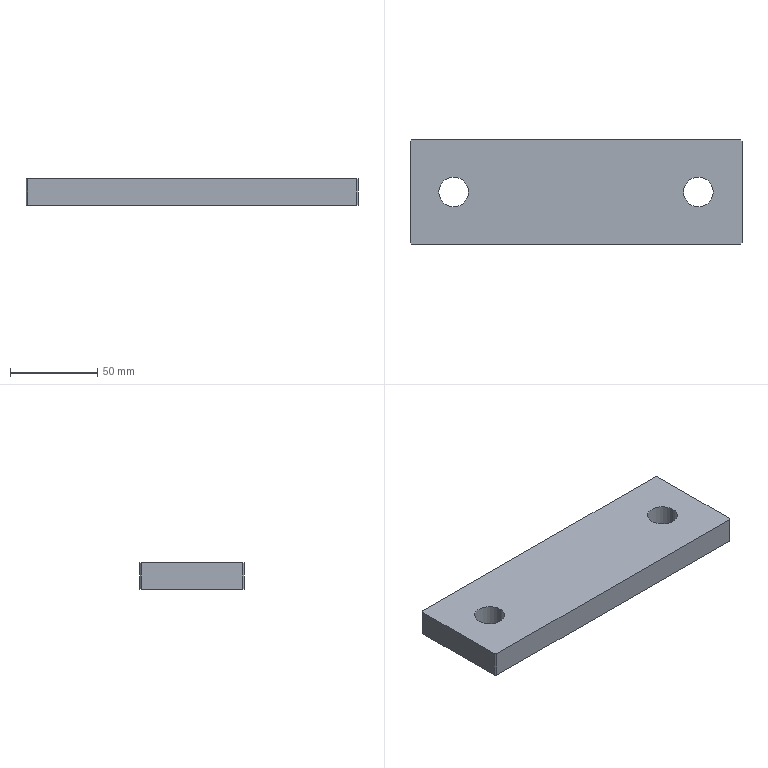Part | STEP file | Reinforcing plate | 1 solid | 14 faces | box 190 x 60 x 15 mm | volume 164161 mm3 | plane 10 | cylinder 4 | commonest cylinder face diameters 17 x4
STEP:
#1=CARTESIAN_POINT('',(0.,0.,0.));
#2=DIRECTION('',(0.,0.,1.));
#3=DIRECTION('',(1.,0.,0.));
#4=AXIS2_PLACEMENT_3D('',#1,#2,#3);
#5=CARTESIAN_POINT('',(516.5,-950.,15.));
#6=VERTEX_POINT('',#5);
#7=CARTESIAN_POINT('',(516.5,-950.,0.));
#8=VERTEX_POINT('',#7);
#9=CARTESIAN_POINT('',(516.5,-950.,0.));
#10=DIRECTION('',(0.,0.,-1.));
#11=VECTOR('',#10,1.);
#12=LINE('',#9,#11);
#13=CARTESIAN_POINT('',(525.,-950.,0.));
#14=DIRECTION('',(0.,0.,-1.));
#15=DIRECTION('',(-1.,0.,0.));
#16=AXIS2_PLACEMENT_3D('',#13,#14,#15);
#17=CYLINDRICAL_SURFACE('',#16,8.5);
#18=CARTESIAN_POINT('',(6.283,0.));
#19=DIRECTION('',(0.,1.));
#20=VECTOR('',#19,1.);
#21=LINE('',#18,#20);
#22=(GEOMETRIC_REPRESENTATION_CONTEXT(2)PARAMETRIC_REPRESENTATION_CONTEXT()REPRESENTATION_CONTEXT('',''));
#23=DEFINITIONAL_REPRESENTATION('',(#21),#22);
#24=PCURVE('',#17,#23);
#25=CARTESIAN_POINT('',(525.,-950.,0.));
#26=DIRECTION('',(0.,0.,-1.));
#27=DIRECTION('',(-1.,0.,0.));
#28=AXIS2_PLACEMENT_3D('',#25,#26,#27);
#29=CYLINDRICAL_SURFACE('',#28,8.5);
#30=CARTESIAN_POINT('',(0.,0.));
#31=DIRECTION('',(0.,1.));
#32=VECTOR('',#31,1.);
#33=LINE('',#30,#32);
#34=(GEOMETRIC_REPRESENTATION_CONTEXT(2)PARAMETRIC_REPRESENTATION_CONTEXT()REPRESENTATION_CONTEXT('',''));
#35=DEFINITIONAL_REPRESENTATION('',(#33),#34);
#36=PCURVE('',#29,#35);
#37=SURFACE_CURVE('',#12,(#24,#36),.PCURVE_S1.);
#38=EDGE_CURVE('',#6,#8,#37,.T.);
#39=ORIENTED_EDGE('',*,*,#38,.T.);
#40=CARTESIAN_POINT('',(533.5,-950.,0.));
#41=VERTEX_POINT('',#40);
#42=CARTESIAN_POINT('',(525.,-950.,0.));
#43=DIRECTION('',(0.,0.,-1.));
#44=DIRECTION('',(-1.,0.,0.));
#45=AXIS2_PLACEMENT_3D('',#42,#43,#44);
#46=CIRCLE('',#45,8.5);
#47=CARTESIAN_POINT('',(0.,0.));
#48=DIRECTION('',(1.,0.));
#49=VECTOR('',#48,1.);
#50=LINE('',#47,#49);
#51=(GEOMETRIC_REPRESENTATION_CONTEXT(2)PARAMETRIC_REPRESENTATION_CONTEXT()REPRESENTATION_CONTEXT('',''));
#52=DEFINITIONAL_REPRESENTATION('',(#50),#51);
#53=PCURVE('',#17,#52);
#54=CARTESIAN_POINT('',(0.,0.,0.));
#55=DIRECTION('',(0.,0.,1.));
#56=DIRECTION('',(1.,0.,0.));
#57=AXIS2_PLACEMENT_3D('',#54,#55,#56);
#58=PLANE('',#57);
#59=CARTESIAN_POINT('',(516.5,-950.));
#60=CARTESIAN_POINT('',(516.5,-935.278));
#61=CARTESIAN_POINT('',(529.25,-942.639));
#62=CARTESIAN_POINT('',(542.,-950.));
#63=CARTESIAN_POINT('',(529.25,-957.361));
#64=CARTESIAN_POINT('',(516.5,-964.722));
#65=CARTESIAN_POINT('',(516.5,-950.));
#66=(BOUNDED_CURVE()B_SPLINE_CURVE(2,(#59,#60,#61,#62,#63,#64,#65),.UNSPECIFIED.,.T.,.F.)B_SPLINE_CURVE_WITH_KNOTS((1,2,2,2,2,1),(-2.094,0.,2.094,4.189,6.283,8.378),.UNSPECIFIED.)CURVE()GEOMETRIC_REPRESENTATION_ITEM()RATIONAL_B_SPLINE_CURVE((1.,0.5,1.,0.5,1.,0.5,1.))REPRESENTATION_ITEM(''));
#67=(GEOMETRIC_REPRESENTATION_CONTEXT(2)PARAMETRIC_REPRESENTATION_CONTEXT()REPRESENTATION_CONTEXT('',''));
#68=DEFINITIONAL_REPRESENTATION('',(#66),#67);
#69=PCURVE('',#58,#68);
#70=SURFACE_CURVE('',#46,(#53,#69),.PCURVE_S1.);
#71=EDGE_CURVE('',#41,#8,#70,.T.);
#72=ORIENTED_EDGE('',*,*,#71,.F.);
#73=CARTESIAN_POINT('',(533.5,-950.,15.));
#74=VERTEX_POINT('',#73);
#75=CARTESIAN_POINT('',(533.5,-950.,0.));
#76=DIRECTION('',(0.,0.,-1.));
#77=VECTOR('',#76,1.);
#78=LINE('',#75,#77);
#79=CARTESIAN_POINT('',(3.142,0.));
#80=DIRECTION('',(0.,1.));
#81=VECTOR('',#80,1.);
#82=LINE('',#79,#81);
#83=(GEOMETRIC_REPRESENTATION_CONTEXT(2)PARAMETRIC_REPRESENTATION_CONTEXT()REPRESENTATION_CONTEXT('',''));
#84=DEFINITIONAL_REPRESENTATION('',(#82),#83);
#85=PCURVE('',#17,#84);
#86=CARTESIAN_POINT('',(3.142,0.));
#87=DIRECTION('',(0.,1.));
#88=VECTOR('',#87,1.);
#89=LINE('',#86,#88);
#90=(GEOMETRIC_REPRESENTATION_CONTEXT(2)PARAMETRIC_REPRESENTATION_CONTEXT()REPRESENTATION_CONTEXT('',''));
#91=DEFINITIONAL_REPRESENTATION('',(#89),#90);
#92=PCURVE('',#29,#91);
#93=SURFACE_CURVE('',#78,(#85,#92),.PCURVE_S1.);
#94=EDGE_CURVE('',#74,#41,#93,.T.);
#95=ORIENTED_EDGE('',*,*,#94,.F.);
#96=CARTESIAN_POINT('',(525.,-950.,15.));
#97=DIRECTION('',(0.,0.,-1.));
#98=DIRECTION('',(-1.,0.,0.));
#99=AXIS2_PLACEMENT_3D('',#96,#97,#98);
#100=CIRCLE('',#99,8.5);
#101=CARTESIAN_POINT('',(0.,-15.));
#102=DIRECTION('',(1.,0.));
#103=VECTOR('',#102,1.);
#104=LINE('',#101,#103);
#105=(GEOMETRIC_REPRESENTATION_CONTEXT(2)PARAMETRIC_REPRESENTATION_CONTEXT()REPRESENTATION_CONTEXT('',''));
#106=DEFINITIONAL_REPRESENTATION('',(#104),#105);
#107=PCURVE('',#17,#106);
#108=CARTESIAN_POINT('',(0.,0.,15.));
#109=DIRECTION('',(0.,0.,1.));
#110=DIRECTION('',(1.,0.,0.));
#111=AXIS2_PLACEMENT_3D('',#108,#109,#110);
#112=PLANE('',#111);
#113=CARTESIAN_POINT('',(516.5,-950.));
#114=CARTESIAN_POINT('',(516.5,-935.278));
#115=CARTESIAN_POINT('',(529.25,-942.639));
#116=CARTESIAN_POINT('',(542.,-950.));
#117=CARTESIAN_POINT('',(529.25,-957.361));
#118=CARTESIAN_POINT('',(516.5,-964.722));
#119=CARTESIAN_POINT('',(516.5,-950.));
#120=(BOUNDED_CURVE()B_SPLINE_CURVE(2,(#113,#114,#115,#116,#117,#118,#119),.UNSPECIFIED.,.T.,.F.)B_SPLINE_CURVE_WITH_KNOTS((1,2,2,2,2,1),(-2.094,0.,2.094,4.189,6.283,8.378),.UNSPECIFIED.)CURVE()GEOMETRIC_REPRESENTATION_ITEM()RATIONAL_B_SPLINE_CURVE((1.,0.5,1.,0.5,1.,0.5,1.))REPRESENTATION_ITEM(''));
#121=(GEOMETRIC_REPRESENTATION_CONTEXT(2)PARAMETRIC_REPRESENTATION_CONTEXT()REPRESENTATION_CONTEXT('',''));
#122=DEFINITIONAL_REPRESENTATION('',(#120),#121);
#123=PCURVE('',#112,#122);
#124=SURFACE_CURVE('',#100,(#107,#123),.PCURVE_S1.);
#125=EDGE_CURVE('',#74,#6,#124,.T.);
#126=ORIENTED_EDGE('',*,*,#125,.T.);
#127=EDGE_LOOP('',(#39,#72,#95,#126));
#128=FACE_BOUND('',#127,.F.);
#129=ADVANCED_FACE('',(#128),#17,.F.);
#130=CARTESIAN_POINT('',(376.5,-950.,15.));
#131=VERTEX_POINT('',#130);
#132=CARTESIAN_POINT('',(376.5,-950.,0.));
#133=VERTEX_POINT('',#132);
#134=CARTESIAN_POINT('',(376.5,-950.,0.));
#135=DIRECTION('',(0.,0.,-1.));
#136=VECTOR('',#135,1.);
#137=LINE('',#134,#136);
#138=CARTESIAN_POINT('',(385.,-950.,0.));
#139=DIRECTION('',(0.,0.,-1.));
#140=DIRECTION('',(-1.,0.,0.));
#141=AXIS2_PLACEMENT_3D('',#138,#139,#140);
#142=CYLINDRICAL_SURFACE('',#141,8.5);
#143=CARTESIAN_POINT('',(6.283,0.));
#144=DIRECTION('',(0.,1.));
#145=VECTOR('',#144,1.);
#146=LINE('',#143,#145);
#147=(GEOMETRIC_REPRESENTATION_CONTEXT(2)PARAMETRIC_REPRESENTATION_CONTEXT()REPRESENTATION_CONTEXT('',''));
#148=DEFINITIONAL_REPRESENTATION('',(#146),#147);
#149=PCURVE('',#142,#148);
#150=CARTESIAN_POINT('',(385.,-950.,0.));
#151=DIRECTION('',(0.,0.,-1.));
#152=DIRECTION('',(-1.,0.,0.));
#153=AXIS2_PLACEMENT_3D('',#150,#151,#152);
#154=CYLINDRICAL_SURFACE('',#153,8.5);
#155=CARTESIAN_POINT('',(0.,0.));
#156=DIRECTION('',(0.,1.));
#157=VECTOR('',#156,1.);
#158=LINE('',#155,#157);
#159=(GEOMETRIC_REPRESENTATION_CONTEXT(2)PARAMETRIC_REPRESENTATION_CONTEXT()REPRESENTATION_CONTEXT('',''));
#160=DEFINITIONAL_REPRESENTATION('',(#158),#159);
#161=PCURVE('',#154,#160);
#162=SURFACE_CURVE('',#137,(#149,#161),.PCURVE_S1.);
#163=EDGE_CURVE('',#131,#133,#162,.T.);
#164=ORIENTED_EDGE('',*,*,#163,.T.);
#165=CARTESIAN_POINT('',(393.5,-950.,0.));
#166=VERTEX_POINT('',#165);
#167=CARTESIAN_POINT('',(385.,-950.,0.));
#168=DIRECTION('',(0.,0.,-1.));
#169=DIRECTION('',(-1.,0.,0.));
#170=AXIS2_PLACEMENT_3D('',#167,#168,#169);
#171=CIRCLE('',#170,8.5);
#172=CARTESIAN_POINT('',(0.,0.));
#173=DIRECTION('',(1.,0.));
#174=VECTOR('',#173,1.);
#175=LINE('',#172,#174);
#176=(GEOMETRIC_REPRESENTATION_CONTEXT(2)PARAMETRIC_REPRESENTATION_CONTEXT()REPRESENTATION_CONTEXT('',''));
#177=DEFINITIONAL_REPRESENTATION('',(#175),#176);
#178=PCURVE('',#142,#177);
#179=CARTESIAN_POINT('',(376.5,-950.));
#180=CARTESIAN_POINT('',(376.5,-935.278));
#181=CARTESIAN_POINT('',(389.25,-942.639));
#182=CARTESIAN_POINT('',(402.,-950.));
#183=CARTESIAN_POINT('',(389.25,-957.361));
#184=CARTESIAN_POINT('',(376.5,-964.722));
#185=CARTESIAN_POINT('',(376.5,-950.));
#186=(BOUNDED_CURVE()B_SPLINE_CURVE(2,(#179,#180,#181,#182,#183,#184,#185),.UNSPECIFIED.,.T.,.F.)B_SPLINE_CURVE_WITH_KNOTS((1,2,2,2,2,1),(-2.094,0.,2.094,4.189,6.283,8.378),.UNSPECIFIED.)CURVE()GEOMETRIC_REPRESENTATION_ITEM()RATIONAL_B_SPLINE_CURVE((1.,0.5,1.,0.5,1.,0.5,1.))REPRESENTATION_ITEM(''));
#187=(GEOMETRIC_REPRESENTATION_CONTEXT(2)PARAMETRIC_REPRESENTATION_CONTEXT()REPRESENTATION_CONTEXT('',''));
#188=DEFINITIONAL_REPRESENTATION('',(#186),#187);
#189=PCURVE('',#58,#188);
#190=SURFACE_CURVE('',#171,(#178,#189),.PCURVE_S1.);
#191=EDGE_CURVE('',#166,#133,#190,.T.);
#192=ORIENTED_EDGE('',*,*,#191,.F.);
#193=CARTESIAN_POINT('',(393.5,-950.,15.));
#194=VERTEX_POINT('',#193);
#195=CARTESIAN_POINT('',(393.5,-950.,0.));
#196=DIRECTION('',(0.,0.,-1.));
#197=VECTOR('',#196,1.);
#198=LINE('',#195,#197);
#199=CARTESIAN_POINT('',(3.142,0.));
#200=DIRECTION('',(0.,1.));
#201=VECTOR('',#200,1.);
#202=LINE('',#199,#201);
#203=(GEOMETRIC_REPRESENTATION_CONTEXT(2)PARAMETRIC_REPRESENTATION_CONTEXT()REPRESENTATION_CONTEXT('',''));
#204=DEFINITIONAL_REPRESENTATION('',(#202),#203);
#205=PCURVE('',#142,#204);
#206=CARTESIAN_POINT('',(3.142,0.));
#207=DIRECTION('',(0.,1.));
#208=VECTOR('',#207,1.);
#209=LINE('',#206,#208);
#210=(GEOMETRIC_REPRESENTATION_CONTEXT(2)PARAMETRIC_REPRESENTATION_CONTEXT()REPRESENTATION_CONTEXT('',''));
#211=DEFINITIONAL_REPRESENTATION('',(#209),#210);
#212=PCURVE('',#154,#211);
#213=SURFACE_CURVE('',#198,(#205,#212),.PCURVE_S1.);
#214=EDGE_CURVE('',#194,#166,#213,.T.);
#215=ORIENTED_EDGE('',*,*,#214,.F.);
#216=CARTESIAN_POINT('',(385.,-950.,15.));
#217=DIRECTION('',(0.,0.,-1.));
#218=DIRECTION('',(-1.,0.,0.));
#219=AXIS2_PLACEMENT_3D('',#216,#217,#218);
#220=CIRCLE('',#219,8.5);
#221=CARTESIAN_POINT('',(0.,-15.));
#222=DIRECTION('',(1.,0.));
#223=VECTOR('',#222,1.);
#224=LINE('',#221,#223);
#225=(GEOMETRIC_REPRESENTATION_CONTEXT(2)PARAMETRIC_REPRESENTATION_CONTEXT()REPRESENTATION_CONTEXT('',''));
#226=DEFINITIONAL_REPRESENTATION('',(#224),#225);
#227=PCURVE('',#142,#226);
#228=CARTESIAN_POINT('',(376.5,-950.));
#229=CARTESIAN_POINT('',(376.5,-935.278));
#230=CARTESIAN_POINT('',(389.25,-942.639));
#231=CARTESIAN_POINT('',(402.,-950.));
#232=CARTESIAN_POINT('',(389.25,-957.361));
#233=CARTESIAN_POINT('',(376.5,-964.722));
#234=CARTESIAN_POINT('',(376.5,-950.));
#235=(BOUNDED_CURVE()B_SPLINE_CURVE(2,(#228,#229,#230,#231,#232,#233,#234),.UNSPECIFIED.,.T.,.F.)B_SPLINE_CURVE_WITH_KNOTS((1,2,2,2,2,1),(-2.094,0.,2.094,4.189,6.283,8.378),.UNSPECIFIED.)CURVE()GEOMETRIC_REPRESENTATION_ITEM()RATIONAL_B_SPLINE_CURVE((1.,0.5,1.,0.5,1.,0.5,1.))REPRESENTATION_ITEM(''));
#236=(GEOMETRIC_REPRESENTATION_CONTEXT(2)PARAMETRIC_REPRESENTATION_CONTEXT()REPRESENTATION_CONTEXT('',''));
#237=DEFINITIONAL_REPRESENTATION('',(#235),#236);
#238=PCURVE('',#112,#237);
#239=SURFACE_CURVE('',#220,(#227,#238),.PCURVE_S1.);
#240=EDGE_CURVE('',#194,#131,#239,.T.);
#241=ORIENTED_EDGE('',*,*,#240,.T.);
#242=EDGE_LOOP('',(#164,#192,#215,#241));
#243=FACE_BOUND('',#242,.F.);
#244=ADVANCED_FACE('',(#243),#142,.F.);
#245=CARTESIAN_POINT('',(360.,-921.,0.));
#246=VERTEX_POINT('',#245);
#247=CARTESIAN_POINT('',(360.,-979.,0.));
#248=VERTEX_POINT('',#247);
#249=CARTESIAN_POINT('',(360.,-980.,0.));
#250=DIRECTION('',(0.,-1.,0.));
#251=VECTOR('',#250,1.);
#252=LINE('',#249,#251);
#253=CARTESIAN_POINT('',(360.,-980.,15.));
#254=DIRECTION('',(1.,0.,0.));
#255=DIRECTION('',(0.,0.,-1.));
#256=AXIS2_PLACEMENT_3D('',#253,#254,#255);
#257=PLANE('',#256);
#258=CARTESIAN_POINT('',(15.,0.));
#259=DIRECTION('',(0.,-1.));
#260=VECTOR('',#259,1.);
#261=LINE('',#258,#260);
#262=(GEOMETRIC_REPRESENTATION_CONTEXT(2)PARAMETRIC_REPRESENTATION_CONTEXT()REPRESENTATION_CONTEXT('',''));
#263=DEFINITIONAL_REPRESENTATION('',(#261),#262);
#264=PCURVE('',#257,#263);
#265=CARTESIAN_POINT('',(360.,-980.));
#266=DIRECTION('',(0.,-1.));
#267=VECTOR('',#266,1.);
#268=LINE('',#265,#267);
#269=(GEOMETRIC_REPRESENTATION_CONTEXT(2)PARAMETRIC_REPRESENTATION_CONTEXT()REPRESENTATION_CONTEXT('',''));
#270=DEFINITIONAL_REPRESENTATION('',(#268),#269);
#271=PCURVE('',#58,#270);
#272=SURFACE_CURVE('',#252,(#264,#271),.PCURVE_S1.);
#273=EDGE_CURVE('',#246,#248,#272,.T.);
#274=ORIENTED_EDGE('',*,*,#273,.T.);
#275=CARTESIAN_POINT('',(360.,-979.,15.));
#276=VERTEX_POINT('',#275);
#277=CARTESIAN_POINT('',(360.,-979.,15.));
#278=DIRECTION('',(0.,0.,1.));
#279=VECTOR('',#278,1.);
#280=LINE('',#277,#279);
#281=CARTESIAN_POINT('',(0.,1.));
#282=DIRECTION('',(-1.,0.));
#283=VECTOR('',#282,1.);
#284=LINE('',#281,#283);
#285=(GEOMETRIC_REPRESENTATION_CONTEXT(2)PARAMETRIC_REPRESENTATION_CONTEXT()REPRESENTATION_CONTEXT('',''));
#286=DEFINITIONAL_REPRESENTATION('',(#284),#285);
#287=PCURVE('',#257,#286);
#288=CARTESIAN_POINT('',(361.,-980.,15.));
#289=DIRECTION('',(0.7071,0.7071,0.));
#290=DIRECTION('',(0.,0.,-1.));
#291=AXIS2_PLACEMENT_3D('',#288,#289,#290);
#292=PLANE('',#291);
#293=CARTESIAN_POINT('',(0.,1.414));
#294=DIRECTION('',(-1.,0.));
#295=VECTOR('',#294,1.);
#296=LINE('',#293,#295);
#297=(GEOMETRIC_REPRESENTATION_CONTEXT(2)PARAMETRIC_REPRESENTATION_CONTEXT()REPRESENTATION_CONTEXT('',''));
#298=DEFINITIONAL_REPRESENTATION('',(#296),#297);
#299=PCURVE('',#292,#298);
#300=SURFACE_CURVE('',#280,(#287,#299),.PCURVE_S1.);
#301=EDGE_CURVE('',#248,#276,#300,.T.);
#302=ORIENTED_EDGE('',*,*,#301,.T.);
#303=CARTESIAN_POINT('',(360.,-921.,15.));
#304=VERTEX_POINT('',#303);
#305=CARTESIAN_POINT('',(360.,-980.,15.));
#306=DIRECTION('',(0.,-1.,0.));
#307=VECTOR('',#306,1.);
#308=LINE('',#305,#307);
#309=CARTESIAN_POINT('',(0.,0.));
#310=DIRECTION('',(0.,-1.));
#311=VECTOR('',#310,1.);
#312=LINE('',#309,#311);
#313=(GEOMETRIC_REPRESENTATION_CONTEXT(2)PARAMETRIC_REPRESENTATION_CONTEXT()REPRESENTATION_CONTEXT('',''));
#314=DEFINITIONAL_REPRESENTATION('',(#312),#313);
#315=PCURVE('',#257,#314);
#316=CARTESIAN_POINT('',(360.,-980.));
#317=DIRECTION('',(0.,-1.));
#318=VECTOR('',#317,1.);
#319=LINE('',#316,#318);
#320=(GEOMETRIC_REPRESENTATION_CONTEXT(2)PARAMETRIC_REPRESENTATION_CONTEXT()REPRESENTATION_CONTEXT('',''));
#321=DEFINITIONAL_REPRESENTATION('',(#319),#320);
#322=PCURVE('',#112,#321);
#323=SURFACE_CURVE('',#308,(#315,#322),.PCURVE_S1.);
#324=EDGE_CURVE('',#304,#276,#323,.T.);
#325=ORIENTED_EDGE('',*,*,#324,.F.);
#326=CARTESIAN_POINT('',(360.,-921.,15.));
#327=DIRECTION('',(0.,0.,-1.));
#328=VECTOR('',#327,1.);
#329=LINE('',#326,#328);
#330=CARTESIAN_POINT('',(0.,59.));
#331=DIRECTION('',(1.,0.));
#332=VECTOR('',#331,1.);
#333=LINE('',#330,#332);
#334=(GEOMETRIC_REPRESENTATION_CONTEXT(2)PARAMETRIC_REPRESENTATION_CONTEXT()REPRESENTATION_CONTEXT('',''));
#335=DEFINITIONAL_REPRESENTATION('',(#333),#334);
#336=PCURVE('',#257,#335);
#337=CARTESIAN_POINT('',(360.,-921.,15.));
#338=DIRECTION('',(0.7071,-0.7071,0.));
#339=DIRECTION('',(0.,0.,-1.));
#340=AXIS2_PLACEMENT_3D('',#337,#338,#339);
#341=PLANE('',#340);
#342=CARTESIAN_POINT('',(0.,0.));
#343=DIRECTION('',(1.,0.));
#344=VECTOR('',#343,1.);
#345=LINE('',#342,#344);
#346=(GEOMETRIC_REPRESENTATION_CONTEXT(2)PARAMETRIC_REPRESENTATION_CONTEXT()REPRESENTATION_CONTEXT('',''));
#347=DEFINITIONAL_REPRESENTATION('',(#345),#346);
#348=PCURVE('',#341,#347);
#349=SURFACE_CURVE('',#329,(#336,#348),.PCURVE_S1.);
#350=EDGE_CURVE('',#304,#246,#349,.T.);
#351=ORIENTED_EDGE('',*,*,#350,.T.);
#352=EDGE_LOOP('',(#274,#302,#325,#351));
#353=FACE_BOUND('',#352,.T.);
#354=ADVANCED_FACE('',(#353),#257,.F.);
#355=CARTESIAN_POINT('',(361.,-980.,0.));
#356=VERTEX_POINT('',#355);
#357=CARTESIAN_POINT('',(549.,-980.,0.));
#358=VERTEX_POINT('',#357);
#359=CARTESIAN_POINT('',(550.,-980.,0.));
#360=DIRECTION('',(1.,0.,0.));
#361=VECTOR('',#360,1.);
#362=LINE('',#359,#361);
#363=CARTESIAN_POINT('',(550.,-980.,15.));
#364=DIRECTION('',(0.,1.,0.));
#365=DIRECTION('',(0.,0.,1.));
#366=AXIS2_PLACEMENT_3D('',#363,#364,#365);
#367=PLANE('',#366);
#368=CARTESIAN_POINT('',(-15.,0.));
#369=DIRECTION('',(0.,1.));
#370=VECTOR('',#369,1.);
#371=LINE('',#368,#370);
#372=(GEOMETRIC_REPRESENTATION_CONTEXT(2)PARAMETRIC_REPRESENTATION_CONTEXT()REPRESENTATION_CONTEXT('',''));
#373=DEFINITIONAL_REPRESENTATION('',(#371),#372);
#374=PCURVE('',#367,#373);
#375=CARTESIAN_POINT('',(550.,-980.));
#376=DIRECTION('',(1.,0.));
#377=VECTOR('',#376,1.);
#378=LINE('',#375,#377);
#379=(GEOMETRIC_REPRESENTATION_CONTEXT(2)PARAMETRIC_REPRESENTATION_CONTEXT()REPRESENTATION_CONTEXT('',''));
#380=DEFINITIONAL_REPRESENTATION('',(#378),#379);
#381=PCURVE('',#58,#380);
#382=SURFACE_CURVE('',#362,(#374,#381),.PCURVE_S1.);
#383=EDGE_CURVE('',#356,#358,#382,.T.);
#384=ORIENTED_EDGE('',*,*,#383,.T.);
#385=CARTESIAN_POINT('',(549.,-980.,15.));
#386=VERTEX_POINT('',#385);
#387=CARTESIAN_POINT('',(549.,-980.,15.));
#388=DIRECTION('',(0.,0.,1.));
#389=VECTOR('',#388,1.);
#390=LINE('',#387,#389);
#391=CARTESIAN_POINT('',(0.,-1.));
#392=DIRECTION('',(1.,0.));
#393=VECTOR('',#392,1.);
#394=LINE('',#391,#393);
#395=(GEOMETRIC_REPRESENTATION_CONTEXT(2)PARAMETRIC_REPRESENTATION_CONTEXT()REPRESENTATION_CONTEXT('',''));
#396=DEFINITIONAL_REPRESENTATION('',(#394),#395);
#397=PCURVE('',#367,#396);
#398=CARTESIAN_POINT('',(550.,-979.,15.));
#399=DIRECTION('',(-0.7071,0.7071,0.));
#400=DIRECTION('',(0.,0.,-1.));
#401=AXIS2_PLACEMENT_3D('',#398,#399,#400);
#402=PLANE('',#401);
#403=CARTESIAN_POINT('',(0.,1.414));
#404=DIRECTION('',(-1.,0.));
#405=VECTOR('',#404,1.);
#406=LINE('',#403,#405);
#407=(GEOMETRIC_REPRESENTATION_CONTEXT(2)PARAMETRIC_REPRESENTATION_CONTEXT()REPRESENTATION_CONTEXT('',''));
#408=DEFINITIONAL_REPRESENTATION('',(#406),#407);
#409=PCURVE('',#402,#408);
#410=SURFACE_CURVE('',#390,(#397,#409),.PCURVE_S1.);
#411=EDGE_CURVE('',#358,#386,#410,.T.);
#412=ORIENTED_EDGE('',*,*,#411,.T.);
#413=CARTESIAN_POINT('',(361.,-980.,15.));
#414=VERTEX_POINT('',#413);
#415=CARTESIAN_POINT('',(550.,-980.,15.));
#416=DIRECTION('',(1.,0.,0.));
#417=VECTOR('',#416,1.);
#418=LINE('',#415,#417);
#419=CARTESIAN_POINT('',(0.,0.));
#420=DIRECTION('',(0.,1.));
#421=VECTOR('',#420,1.);
#422=LINE('',#419,#421);
#423=(GEOMETRIC_REPRESENTATION_CONTEXT(2)PARAMETRIC_REPRESENTATION_CONTEXT()REPRESENTATION_CONTEXT('',''));
#424=DEFINITIONAL_REPRESENTATION('',(#422),#423);
#425=PCURVE('',#367,#424);
#426=CARTESIAN_POINT('',(550.,-980.));
#427=DIRECTION('',(1.,0.));
#428=VECTOR('',#427,1.);
#429=LINE('',#426,#428);
#430=(GEOMETRIC_REPRESENTATION_CONTEXT(2)PARAMETRIC_REPRESENTATION_CONTEXT()REPRESENTATION_CONTEXT('',''));
#431=DEFINITIONAL_REPRESENTATION('',(#429),#430);
#432=PCURVE('',#112,#431);
#433=SURFACE_CURVE('',#418,(#425,#432),.PCURVE_S1.);
#434=EDGE_CURVE('',#414,#386,#433,.T.);
#435=ORIENTED_EDGE('',*,*,#434,.F.);
#436=CARTESIAN_POINT('',(361.,-980.,15.));
#437=DIRECTION('',(0.,0.,-1.));
#438=VECTOR('',#437,1.);
#439=LINE('',#436,#438);
#440=CARTESIAN_POINT('',(0.,-189.));
#441=DIRECTION('',(-1.,0.));
#442=VECTOR('',#441,1.);
#443=LINE('',#440,#442);
#444=(GEOMETRIC_REPRESENTATION_CONTEXT(2)PARAMETRIC_REPRESENTATION_CONTEXT()REPRESENTATION_CONTEXT('',''));
#445=DEFINITIONAL_REPRESENTATION('',(#443),#444);
#446=PCURVE('',#367,#445);
#447=CARTESIAN_POINT('',(0.,0.));
#448=DIRECTION('',(1.,0.));
#449=VECTOR('',#448,1.);
#450=LINE('',#447,#449);
#451=(GEOMETRIC_REPRESENTATION_CONTEXT(2)PARAMETRIC_REPRESENTATION_CONTEXT()REPRESENTATION_CONTEXT('',''));
#452=DEFINITIONAL_REPRESENTATION('',(#450),#451);
#453=PCURVE('',#292,#452);
#454=SURFACE_CURVE('',#439,(#446,#453),.PCURVE_S1.);
#455=EDGE_CURVE('',#414,#356,#454,.T.);
#456=ORIENTED_EDGE('',*,*,#455,.T.);
#457=EDGE_LOOP('',(#384,#412,#435,#456));
#458=FACE_BOUND('',#457,.T.);
#459=ADVANCED_FACE('',(#458),#367,.F.);
#460=CARTESIAN_POINT('',(550.,-979.,15.));
#461=VERTEX_POINT('',#460);
#462=CARTESIAN_POINT('',(550.,-921.,15.));
#463=VERTEX_POINT('',#462);
#464=CARTESIAN_POINT('',(550.,-980.,15.));
#465=DIRECTION('',(0.,1.,0.));
#466=VECTOR('',#465,1.);
#467=LINE('',#464,#466);
#468=CARTESIAN_POINT('',(550.,-980.,15.));
#469=DIRECTION('',(-1.,0.,0.));
#470=DIRECTION('',(0.,0.,1.));
#471=AXIS2_PLACEMENT_3D('',#468,#469,#470);
#472=PLANE('',#471);
#473=CARTESIAN_POINT('',(0.,0.));
#474=DIRECTION('',(0.,1.));
#475=VECTOR('',#474,1.);
#476=LINE('',#473,#475);
#477=(GEOMETRIC_REPRESENTATION_CONTEXT(2)PARAMETRIC_REPRESENTATION_CONTEXT()REPRESENTATION_CONTEXT('',''));
#478=DEFINITIONAL_REPRESENTATION('',(#476),#477);
#479=PCURVE('',#472,#478);
#480=CARTESIAN_POINT('',(550.,-980.));
#481=DIRECTION('',(0.,1.));
#482=VECTOR('',#481,1.);
#483=LINE('',#480,#482);
#484=(GEOMETRIC_REPRESENTATION_CONTEXT(2)PARAMETRIC_REPRESENTATION_CONTEXT()REPRESENTATION_CONTEXT('',''));
#485=DEFINITIONAL_REPRESENTATION('',(#483),#484);
#486=PCURVE('',#112,#485);
#487=SURFACE_CURVE('',#467,(#479,#486),.PCURVE_S1.);
#488=EDGE_CURVE('',#461,#463,#487,.T.);
#489=ORIENTED_EDGE('',*,*,#488,.F.);
#490=CARTESIAN_POINT('',(550.,-979.,0.));
#491=VERTEX_POINT('',#490);
#492=CARTESIAN_POINT('',(550.,-979.,15.));
#493=DIRECTION('',(0.,0.,-1.));
#494=VECTOR('',#493,1.);
#495=LINE('',#492,#494);
#496=CARTESIAN_POINT('',(0.,1.));
#497=DIRECTION('',(-1.,0.));
#498=VECTOR('',#497,1.);
#499=LINE('',#496,#498);
#500=(GEOMETRIC_REPRESENTATION_CONTEXT(2)PARAMETRIC_REPRESENTATION_CONTEXT()REPRESENTATION_CONTEXT('',''));
#501=DEFINITIONAL_REPRESENTATION('',(#499),#500);
#502=PCURVE('',#472,#501);
#503=CARTESIAN_POINT('',(0.,0.));
#504=DIRECTION('',(1.,0.));
#505=VECTOR('',#504,1.);
#506=LINE('',#503,#505);
#507=(GEOMETRIC_REPRESENTATION_CONTEXT(2)PARAMETRIC_REPRESENTATION_CONTEXT()REPRESENTATION_CONTEXT('',''));
#508=DEFINITIONAL_REPRESENTATION('',(#506),#507);
#509=PCURVE('',#402,#508);
#510=SURFACE_CURVE('',#495,(#502,#509),.PCURVE_S1.);
#511=EDGE_CURVE('',#461,#491,#510,.T.);
#512=ORIENTED_EDGE('',*,*,#511,.T.);
#513=CARTESIAN_POINT('',(550.,-921.,0.));
#514=VERTEX_POINT('',#513);
#515=CARTESIAN_POINT('',(550.,-980.,0.));
#516=DIRECTION('',(0.,1.,0.));
#517=VECTOR('',#516,1.);
#518=LINE('',#515,#517);
#519=CARTESIAN_POINT('',(-15.,0.));
#520=DIRECTION('',(0.,1.));
#521=VECTOR('',#520,1.);
#522=LINE('',#519,#521);
#523=(GEOMETRIC_REPRESENTATION_CONTEXT(2)PARAMETRIC_REPRESENTATION_CONTEXT()REPRESENTATION_CONTEXT('',''));
#524=DEFINITIONAL_REPRESENTATION('',(#522),#523);
#525=PCURVE('',#472,#524);
#526=CARTESIAN_POINT('',(550.,-980.));
#527=DIRECTION('',(0.,1.));
#528=VECTOR('',#527,1.);
#529=LINE('',#526,#528);
#530=(GEOMETRIC_REPRESENTATION_CONTEXT(2)PARAMETRIC_REPRESENTATION_CONTEXT()REPRESENTATION_CONTEXT('',''));
#531=DEFINITIONAL_REPRESENTATION('',(#529),#530);
#532=PCURVE('',#58,#531);
#533=SURFACE_CURVE('',#518,(#525,#532),.PCURVE_S1.);
#534=EDGE_CURVE('',#491,#514,#533,.T.);
#535=ORIENTED_EDGE('',*,*,#534,.T.);
#536=CARTESIAN_POINT('',(550.,-921.,15.));
#537=DIRECTION('',(0.,0.,1.));
#538=VECTOR('',#537,1.);
#539=LINE('',#536,#538);
#540=CARTESIAN_POINT('',(0.,59.));
#541=DIRECTION('',(1.,0.));
#542=VECTOR('',#541,1.);
#543=LINE('',#540,#542);
#544=(GEOMETRIC_REPRESENTATION_CONTEXT(2)PARAMETRIC_REPRESENTATION_CONTEXT()REPRESENTATION_CONTEXT('',''));
#545=DEFINITIONAL_REPRESENTATION('',(#543),#544);
#546=PCURVE('',#472,#545);
#547=CARTESIAN_POINT('',(549.,-920.,15.));
#548=DIRECTION('',(-0.7071,-0.7071,0.));
#549=DIRECTION('',(0.,0.,-1.));
#550=AXIS2_PLACEMENT_3D('',#547,#548,#549);
#551=PLANE('',#550);
#552=CARTESIAN_POINT('',(0.,1.414));
#553=DIRECTION('',(-1.,0.));
#554=VECTOR('',#553,1.);
#555=LINE('',#552,#554);
#556=(GEOMETRIC_REPRESENTATION_CONTEXT(2)PARAMETRIC_REPRESENTATION_CONTEXT()REPRESENTATION_CONTEXT('',''));
#557=DEFINITIONAL_REPRESENTATION('',(#555),#556);
#558=PCURVE('',#551,#557);
#559=SURFACE_CURVE('',#539,(#546,#558),.PCURVE_S1.);
#560=EDGE_CURVE('',#514,#463,#559,.T.);
#561=ORIENTED_EDGE('',*,*,#560,.T.);
#562=EDGE_LOOP('',(#489,#512,#535,#561));
#563=FACE_BOUND('',#562,.T.);
#564=ADVANCED_FACE('',(#563),#472,.F.);
#565=CARTESIAN_POINT('',(549.,-920.,15.));
#566=VERTEX_POINT('',#565);
#567=CARTESIAN_POINT('',(361.,-920.,15.));
#568=VERTEX_POINT('',#567);
#569=CARTESIAN_POINT('',(550.,-920.,15.));
#570=DIRECTION('',(-1.,0.,0.));
#571=VECTOR('',#570,1.);
#572=LINE('',#569,#571);
#573=CARTESIAN_POINT('',(550.,-920.,15.));
#574=DIRECTION('',(0.,-1.,0.));
#575=DIRECTION('',(0.,0.,-1.));
#576=AXIS2_PLACEMENT_3D('',#573,#574,#575);
#577=PLANE('',#576);
#578=CARTESIAN_POINT('',(0.,0.));
#579=DIRECTION('',(0.,-1.));
#580=VECTOR('',#579,1.);
#581=LINE('',#578,#580);
#582=(GEOMETRIC_REPRESENTATION_CONTEXT(2)PARAMETRIC_REPRESENTATION_CONTEXT()REPRESENTATION_CONTEXT('',''));
#583=DEFINITIONAL_REPRESENTATION('',(#581),#582);
#584=PCURVE('',#577,#583);
#585=CARTESIAN_POINT('',(550.,-920.));
#586=DIRECTION('',(-1.,0.));
#587=VECTOR('',#586,1.);
#588=LINE('',#585,#587);
#589=(GEOMETRIC_REPRESENTATION_CONTEXT(2)PARAMETRIC_REPRESENTATION_CONTEXT()REPRESENTATION_CONTEXT('',''));
#590=DEFINITIONAL_REPRESENTATION('',(#588),#589);
#591=PCURVE('',#112,#590);
#592=SURFACE_CURVE('',#572,(#584,#591),.PCURVE_S1.);
#593=EDGE_CURVE('',#566,#568,#592,.T.);
#594=ORIENTED_EDGE('',*,*,#593,.F.);
#595=CARTESIAN_POINT('',(549.,-920.,0.));
#596=VERTEX_POINT('',#595);
#597=CARTESIAN_POINT('',(549.,-920.,15.));
#598=DIRECTION('',(0.,0.,-1.));
#599=VECTOR('',#598,1.);
#600=LINE('',#597,#599);
#601=CARTESIAN_POINT('',(0.,-1.));
#602=DIRECTION('',(1.,0.));
#603=VECTOR('',#602,1.);
#604=LINE('',#601,#603);
#605=(GEOMETRIC_REPRESENTATION_CONTEXT(2)PARAMETRIC_REPRESENTATION_CONTEXT()REPRESENTATION_CONTEXT('',''));
#606=DEFINITIONAL_REPRESENTATION('',(#604),#605);
#607=PCURVE('',#577,#606);
#608=CARTESIAN_POINT('',(0.,0.));
#609=DIRECTION('',(1.,0.));
#610=VECTOR('',#609,1.);
#611=LINE('',#608,#610);
#612=(GEOMETRIC_REPRESENTATION_CONTEXT(2)PARAMETRIC_REPRESENTATION_CONTEXT()REPRESENTATION_CONTEXT('',''));
#613=DEFINITIONAL_REPRESENTATION('',(#611),#612);
#614=PCURVE('',#551,#613);
#615=SURFACE_CURVE('',#600,(#607,#614),.PCURVE_S1.);
#616=EDGE_CURVE('',#566,#596,#615,.T.);
#617=ORIENTED_EDGE('',*,*,#616,.T.);
#618=CARTESIAN_POINT('',(361.,-920.,0.));
#619=VERTEX_POINT('',#618);
#620=CARTESIAN_POINT('',(550.,-920.,0.));
#621=DIRECTION('',(-1.,0.,0.));
#622=VECTOR('',#621,1.);
#623=LINE('',#620,#622);
#624=CARTESIAN_POINT('',(15.,0.));
#625=DIRECTION('',(0.,-1.));
#626=VECTOR('',#625,1.);
#627=LINE('',#624,#626);
#628=(GEOMETRIC_REPRESENTATION_CONTEXT(2)PARAMETRIC_REPRESENTATION_CONTEXT()REPRESENTATION_CONTEXT('',''));
#629=DEFINITIONAL_REPRESENTATION('',(#627),#628);
#630=PCURVE('',#577,#629);
#631=CARTESIAN_POINT('',(550.,-920.));
#632=DIRECTION('',(-1.,0.));
#633=VECTOR('',#632,1.);
#634=LINE('',#631,#633);
#635=(GEOMETRIC_REPRESENTATION_CONTEXT(2)PARAMETRIC_REPRESENTATION_CONTEXT()REPRESENTATION_CONTEXT('',''));
#636=DEFINITIONAL_REPRESENTATION('',(#634),#635);
#637=PCURVE('',#58,#636);
#638=SURFACE_CURVE('',#623,(#630,#637),.PCURVE_S1.);
#639=EDGE_CURVE('',#596,#619,#638,.T.);
#640=ORIENTED_EDGE('',*,*,#639,.T.);
#641=CARTESIAN_POINT('',(361.,-920.,15.));
#642=DIRECTION('',(0.,0.,1.));
#643=VECTOR('',#642,1.);
#644=LINE('',#641,#643);
#645=CARTESIAN_POINT('',(0.,-189.));
#646=DIRECTION('',(-1.,0.));
#647=VECTOR('',#646,1.);
#648=LINE('',#645,#647);
#649=(GEOMETRIC_REPRESENTATION_CONTEXT(2)PARAMETRIC_REPRESENTATION_CONTEXT()REPRESENTATION_CONTEXT('',''));
#650=DEFINITIONAL_REPRESENTATION('',(#648),#649);
#651=PCURVE('',#577,#650);
#652=CARTESIAN_POINT('',(0.,1.414));
#653=DIRECTION('',(-1.,0.));
#654=VECTOR('',#653,1.);
#655=LINE('',#652,#654);
#656=(GEOMETRIC_REPRESENTATION_CONTEXT(2)PARAMETRIC_REPRESENTATION_CONTEXT()REPRESENTATION_CONTEXT('',''));
#657=DEFINITIONAL_REPRESENTATION('',(#655),#656);
#658=PCURVE('',#341,#657);
#659=SURFACE_CURVE('',#644,(#651,#658),.PCURVE_S1.);
#660=EDGE_CURVE('',#619,#568,#659,.T.);
#661=ORIENTED_EDGE('',*,*,#660,.T.);
#662=EDGE_LOOP('',(#594,#617,#640,#661));
#663=FACE_BOUND('',#662,.T.);
#664=ADVANCED_FACE('',(#663),#577,.F.);
#665=CARTESIAN_POINT('',(525.,-950.,15.));
#666=DIRECTION('',(0.,0.,-1.));
#667=DIRECTION('',(-1.,0.,0.));
#668=AXIS2_PLACEMENT_3D('',#665,#666,#667);
#669=CIRCLE('',#668,8.5);
#670=CARTESIAN_POINT('',(516.5,-950.));
#671=CARTESIAN_POINT('',(516.5,-935.278));
#672=CARTESIAN_POINT('',(529.25,-942.639));
#673=CARTESIAN_POINT('',(542.,-950.));
#674=CARTESIAN_POINT('',(529.25,-957.361));
#675=CARTESIAN_POINT('',(516.5,-964.722));
#676=CARTESIAN_POINT('',(516.5,-950.));
#677=(BOUNDED_CURVE()B_SPLINE_CURVE(2,(#670,#671,#672,#673,#674,#675,#676),.UNSPECIFIED.,.T.,.F.)B_SPLINE_CURVE_WITH_KNOTS((1,2,2,2,2,1),(-2.094,0.,2.094,4.189,6.283,8.378),.UNSPECIFIED.)CURVE()GEOMETRIC_REPRESENTATION_ITEM()RATIONAL_B_SPLINE_CURVE((1.,0.5,1.,0.5,1.,0.5,1.))REPRESENTATION_ITEM(''));
#678=(GEOMETRIC_REPRESENTATION_CONTEXT(2)PARAMETRIC_REPRESENTATION_CONTEXT()REPRESENTATION_CONTEXT('',''));
#679=DEFINITIONAL_REPRESENTATION('',(#677),#678);
#680=PCURVE('',#112,#679);
#681=CARTESIAN_POINT('',(0.,-15.));
#682=DIRECTION('',(1.,0.));
#683=VECTOR('',#682,1.);
#684=LINE('',#681,#683);
#685=(GEOMETRIC_REPRESENTATION_CONTEXT(2)PARAMETRIC_REPRESENTATION_CONTEXT()REPRESENTATION_CONTEXT('',''));
#686=DEFINITIONAL_REPRESENTATION('',(#684),#685);
#687=PCURVE('',#29,#686);
#688=SURFACE_CURVE('',#669,(#680,#687),.PCURVE_S1.);
#689=EDGE_CURVE('',#6,#74,#688,.T.);
#690=ORIENTED_EDGE('',*,*,#689,.T.);
#691=ORIENTED_EDGE('',*,*,#125,.T.);
#692=EDGE_LOOP('',(#690,#691));
#693=FACE_BOUND('',#692,.T.);
#694=CARTESIAN_POINT('',(385.,-950.,15.));
#695=DIRECTION('',(0.,0.,-1.));
#696=DIRECTION('',(-1.,0.,0.));
#697=AXIS2_PLACEMENT_3D('',#694,#695,#696);
#698=CIRCLE('',#697,8.5);
#699=CARTESIAN_POINT('',(376.5,-950.));
#700=CARTESIAN_POINT('',(376.5,-935.278));
#701=CARTESIAN_POINT('',(389.25,-942.639));
#702=CARTESIAN_POINT('',(402.,-950.));
#703=CARTESIAN_POINT('',(389.25,-957.361));
#704=CARTESIAN_POINT('',(376.5,-964.722));
#705=CARTESIAN_POINT('',(376.5,-950.));
#706=(BOUNDED_CURVE()B_SPLINE_CURVE(2,(#699,#700,#701,#702,#703,#704,#705),.UNSPECIFIED.,.T.,.F.)B_SPLINE_CURVE_WITH_KNOTS((1,2,2,2,2,1),(-2.094,0.,2.094,4.189,6.283,8.378),.UNSPECIFIED.)CURVE()GEOMETRIC_REPRESENTATION_ITEM()RATIONAL_B_SPLINE_CURVE((1.,0.5,1.,0.5,1.,0.5,1.))REPRESENTATION_ITEM(''));
#707=(GEOMETRIC_REPRESENTATION_CONTEXT(2)PARAMETRIC_REPRESENTATION_CONTEXT()REPRESENTATION_CONTEXT('',''));
#708=DEFINITIONAL_REPRESENTATION('',(#706),#707);
#709=PCURVE('',#112,#708);
#710=CARTESIAN_POINT('',(0.,-15.));
#711=DIRECTION('',(1.,0.));
#712=VECTOR('',#711,1.);
#713=LINE('',#710,#712);
#714=(GEOMETRIC_REPRESENTATION_CONTEXT(2)PARAMETRIC_REPRESENTATION_CONTEXT()REPRESENTATION_CONTEXT('',''));
#715=DEFINITIONAL_REPRESENTATION('',(#713),#714);
#716=PCURVE('',#154,#715);
#717=SURFACE_CURVE('',#698,(#709,#716),.PCURVE_S1.);
#718=EDGE_CURVE('',#131,#194,#717,.T.);
#719=ORIENTED_EDGE('',*,*,#718,.T.);
#720=ORIENTED_EDGE('',*,*,#240,.T.);
#721=EDGE_LOOP('',(#719,#720));
#722=FACE_BOUND('',#721,.T.);
#723=ORIENTED_EDGE('',*,*,#434,.T.);
#724=CARTESIAN_POINT('',(764.5,-764.5,15.));
#725=DIRECTION('',(0.7071,0.7071,0.));
#726=VECTOR('',#725,1.);
#727=LINE('',#724,#726);
#728=CARTESIAN_POINT('',(764.5,-764.5));
#729=DIRECTION('',(0.7071,0.7071));
#730=VECTOR('',#729,1.);
#731=LINE('',#728,#730);
#732=(GEOMETRIC_REPRESENTATION_CONTEXT(2)PARAMETRIC_REPRESENTATION_CONTEXT()REPRESENTATION_CONTEXT('',''));
#733=DEFINITIONAL_REPRESENTATION('',(#731),#732);
#734=PCURVE('',#112,#733);
#735=CARTESIAN_POINT('',(0.,-303.349));
#736=DIRECTION('',(0.,-1.));
#737=VECTOR('',#736,1.);
#738=LINE('',#735,#737);
#739=(GEOMETRIC_REPRESENTATION_CONTEXT(2)PARAMETRIC_REPRESENTATION_CONTEXT()REPRESENTATION_CONTEXT('',''));
#740=DEFINITIONAL_REPRESENTATION('',(#738),#739);
#741=PCURVE('',#402,#740);
#742=SURFACE_CURVE('',#727,(#734,#741),.PCURVE_S1.);
#743=EDGE_CURVE('',#386,#461,#742,.T.);
#744=ORIENTED_EDGE('',*,*,#743,.T.);
#745=ORIENTED_EDGE('',*,*,#488,.T.);
#746=CARTESIAN_POINT('',(-185.5,-185.5,15.));
#747=DIRECTION('',(-0.7071,0.7071,0.));
#748=VECTOR('',#747,1.);
#749=LINE('',#746,#748);
#750=CARTESIAN_POINT('',(-185.5,-185.5));
#751=DIRECTION('',(-0.7071,0.7071));
#752=VECTOR('',#751,1.);
#753=LINE('',#750,#752);
#754=(GEOMETRIC_REPRESENTATION_CONTEXT(2)PARAMETRIC_REPRESENTATION_CONTEXT()REPRESENTATION_CONTEXT('',''));
#755=DEFINITIONAL_REPRESENTATION('',(#753),#754);
#756=PCURVE('',#112,#755);
#757=CARTESIAN_POINT('',(0.,-1038.74));
#758=DIRECTION('',(0.,-1.));
#759=VECTOR('',#758,1.);
#760=LINE('',#757,#759);
#761=(GEOMETRIC_REPRESENTATION_CONTEXT(2)PARAMETRIC_REPRESENTATION_CONTEXT()REPRESENTATION_CONTEXT('',''));
#762=DEFINITIONAL_REPRESENTATION('',(#760),#761);
#763=PCURVE('',#551,#762);
#764=SURFACE_CURVE('',#749,(#756,#763),.PCURVE_S1.);
#765=EDGE_CURVE('',#463,#566,#764,.T.);
#766=ORIENTED_EDGE('',*,*,#765,.T.);
#767=ORIENTED_EDGE('',*,*,#593,.T.);
#768=CARTESIAN_POINT('',(640.5,-640.5,15.));
#769=DIRECTION('',(-0.7071,-0.7071,0.));
#770=VECTOR('',#769,1.);
#771=LINE('',#768,#770);
#772=CARTESIAN_POINT('',(640.5,-640.5));
#773=DIRECTION('',(-0.7071,-0.7071));
#774=VECTOR('',#773,1.);
#775=LINE('',#772,#774);
#776=(GEOMETRIC_REPRESENTATION_CONTEXT(2)PARAMETRIC_REPRESENTATION_CONTEXT()REPRESENTATION_CONTEXT('',''));
#777=DEFINITIONAL_REPRESENTATION('',(#775),#776);
#778=PCURVE('',#112,#777);
#779=CARTESIAN_POINT('',(0.,396.687));
#780=DIRECTION('',(0.,-1.));
#781=VECTOR('',#780,1.);
#782=LINE('',#779,#781);
#783=(GEOMETRIC_REPRESENTATION_CONTEXT(2)PARAMETRIC_REPRESENTATION_CONTEXT()REPRESENTATION_CONTEXT('',''));
#784=DEFINITIONAL_REPRESENTATION('',(#782),#783);
#785=PCURVE('',#341,#784);
#786=SURFACE_CURVE('',#771,(#778,#785),.PCURVE_S1.);
#787=EDGE_CURVE('',#568,#304,#786,.T.);
#788=ORIENTED_EDGE('',*,*,#787,.T.);
#789=ORIENTED_EDGE('',*,*,#324,.T.);
#790=CARTESIAN_POINT('',(-309.5,-309.5,15.));
#791=DIRECTION('',(0.7071,-0.7071,0.));
#792=VECTOR('',#791,1.);
#793=LINE('',#790,#792);
#794=CARTESIAN_POINT('',(-309.5,-309.5));
#795=DIRECTION('',(0.7071,-0.7071));
#796=VECTOR('',#795,1.);
#797=LINE('',#794,#796);
#798=(GEOMETRIC_REPRESENTATION_CONTEXT(2)PARAMETRIC_REPRESENTATION_CONTEXT()REPRESENTATION_CONTEXT('',''));
#799=DEFINITIONAL_REPRESENTATION('',(#797),#798);
#800=PCURVE('',#112,#799);
#801=CARTESIAN_POINT('',(0.,948.23));
#802=DIRECTION('',(0.,-1.));
#803=VECTOR('',#802,1.);
#804=LINE('',#801,#803);
#805=(GEOMETRIC_REPRESENTATION_CONTEXT(2)PARAMETRIC_REPRESENTATION_CONTEXT()REPRESENTATION_CONTEXT('',''));
#806=DEFINITIONAL_REPRESENTATION('',(#804),#805);
#807=PCURVE('',#292,#806);
#808=SURFACE_CURVE('',#793,(#800,#807),.PCURVE_S1.);
#809=EDGE_CURVE('',#276,#414,#808,.T.);
#810=ORIENTED_EDGE('',*,*,#809,.T.);
#811=EDGE_LOOP('',(#723,#744,#745,#766,#767,#788,#789,#810));
#812=FACE_BOUND('',#811,.T.);
#813=ADVANCED_FACE('',(#693,#722,#812),#112,.T.);
#814=CARTESIAN_POINT('',(525.,-950.,0.));
#815=DIRECTION('',(0.,0.,-1.));
#816=DIRECTION('',(-1.,0.,0.));
#817=AXIS2_PLACEMENT_3D('',#814,#815,#816);
#818=CIRCLE('',#817,8.5);
#819=CARTESIAN_POINT('',(516.5,-950.));
#820=CARTESIAN_POINT('',(516.5,-935.278));
#821=CARTESIAN_POINT('',(529.25,-942.639));
#822=CARTESIAN_POINT('',(542.,-950.));
#823=CARTESIAN_POINT('',(529.25,-957.361));
#824=CARTESIAN_POINT('',(516.5,-964.722));
#825=CARTESIAN_POINT('',(516.5,-950.));
#826=(BOUNDED_CURVE()B_SPLINE_CURVE(2,(#819,#820,#821,#822,#823,#824,#825),.UNSPECIFIED.,.T.,.F.)B_SPLINE_CURVE_WITH_KNOTS((1,2,2,2,2,1),(-2.094,0.,2.094,4.189,6.283,8.378),.UNSPECIFIED.)CURVE()GEOMETRIC_REPRESENTATION_ITEM()RATIONAL_B_SPLINE_CURVE((1.,0.5,1.,0.5,1.,0.5,1.))REPRESENTATION_ITEM(''));
#827=(GEOMETRIC_REPRESENTATION_CONTEXT(2)PARAMETRIC_REPRESENTATION_CONTEXT()REPRESENTATION_CONTEXT('',''));
#828=DEFINITIONAL_REPRESENTATION('',(#826),#827);
#829=PCURVE('',#58,#828);
#830=CARTESIAN_POINT('',(0.,0.));
#831=DIRECTION('',(1.,0.));
#832=VECTOR('',#831,1.);
#833=LINE('',#830,#832);
#834=(GEOMETRIC_REPRESENTATION_CONTEXT(2)PARAMETRIC_REPRESENTATION_CONTEXT()REPRESENTATION_CONTEXT('',''));
#835=DEFINITIONAL_REPRESENTATION('',(#833),#834);
#836=PCURVE('',#29,#835);
#837=SURFACE_CURVE('',#818,(#829,#836),.PCURVE_S1.);
#838=EDGE_CURVE('',#8,#41,#837,.T.);
#839=ORIENTED_EDGE('',*,*,#838,.F.);
#840=ORIENTED_EDGE('',*,*,#71,.F.);
#841=EDGE_LOOP('',(#839,#840));
#842=FACE_BOUND('',#841,.T.);
#843=CARTESIAN_POINT('',(385.,-950.,0.));
#844=DIRECTION('',(0.,0.,-1.));
#845=DIRECTION('',(-1.,0.,0.));
#846=AXIS2_PLACEMENT_3D('',#843,#844,#845);
#847=CIRCLE('',#846,8.5);
#848=CARTESIAN_POINT('',(376.5,-950.));
#849=CARTESIAN_POINT('',(376.5,-935.278));
#850=CARTESIAN_POINT('',(389.25,-942.639));
#851=CARTESIAN_POINT('',(402.,-950.));
#852=CARTESIAN_POINT('',(389.25,-957.361));
#853=CARTESIAN_POINT('',(376.5,-964.722));
#854=CARTESIAN_POINT('',(376.5,-950.));
#855=(BOUNDED_CURVE()B_SPLINE_CURVE(2,(#848,#849,#850,#851,#852,#853,#854),.UNSPECIFIED.,.T.,.F.)B_SPLINE_CURVE_WITH_KNOTS((1,2,2,2,2,1),(-2.094,0.,2.094,4.189,6.283,8.378),.UNSPECIFIED.)CURVE()GEOMETRIC_REPRESENTATION_ITEM()RATIONAL_B_SPLINE_CURVE((1.,0.5,1.,0.5,1.,0.5,1.))REPRESENTATION_ITEM(''));
#856=(GEOMETRIC_REPRESENTATION_CONTEXT(2)PARAMETRIC_REPRESENTATION_CONTEXT()REPRESENTATION_CONTEXT('',''));
#857=DEFINITIONAL_REPRESENTATION('',(#855),#856);
#858=PCURVE('',#58,#857);
#859=CARTESIAN_POINT('',(0.,0.));
#860=DIRECTION('',(1.,0.));
#861=VECTOR('',#860,1.);
#862=LINE('',#859,#861);
#863=(GEOMETRIC_REPRESENTATION_CONTEXT(2)PARAMETRIC_REPRESENTATION_CONTEXT()REPRESENTATION_CONTEXT('',''));
#864=DEFINITIONAL_REPRESENTATION('',(#862),#863);
#865=PCURVE('',#154,#864);
#866=SURFACE_CURVE('',#847,(#858,#865),.PCURVE_S1.);
#867=EDGE_CURVE('',#133,#166,#866,.T.);
#868=ORIENTED_EDGE('',*,*,#867,.F.);
#869=ORIENTED_EDGE('',*,*,#191,.F.);
#870=EDGE_LOOP('',(#868,#869));
#871=FACE_BOUND('',#870,.T.);
#872=ORIENTED_EDGE('',*,*,#534,.F.);
#873=CARTESIAN_POINT('',(550.,-979.,0.));
#874=DIRECTION('',(-0.7071,-0.7071,0.));
#875=VECTOR('',#874,1.);
#876=LINE('',#873,#875);
#877=CARTESIAN_POINT('',(550.,-979.));
#878=DIRECTION('',(-0.7071,-0.7071));
#879=VECTOR('',#878,1.);
#880=LINE('',#877,#879);
#881=(GEOMETRIC_REPRESENTATION_CONTEXT(2)PARAMETRIC_REPRESENTATION_CONTEXT()REPRESENTATION_CONTEXT('',''));
#882=DEFINITIONAL_REPRESENTATION('',(#880),#881);
#883=PCURVE('',#58,#882);
#884=CARTESIAN_POINT('',(15.,0.));
#885=DIRECTION('',(0.,1.));
#886=VECTOR('',#885,1.);
#887=LINE('',#884,#886);
#888=(GEOMETRIC_REPRESENTATION_CONTEXT(2)PARAMETRIC_REPRESENTATION_CONTEXT()REPRESENTATION_CONTEXT('',''));
#889=DEFINITIONAL_REPRESENTATION('',(#887),#888);
#890=PCURVE('',#402,#889);
#891=SURFACE_CURVE('',#876,(#883,#890),.PCURVE_S1.);
#892=EDGE_CURVE('',#491,#358,#891,.T.);
#893=ORIENTED_EDGE('',*,*,#892,.T.);
#894=ORIENTED_EDGE('',*,*,#383,.F.);
#895=CARTESIAN_POINT('',(361.,-980.,0.));
#896=DIRECTION('',(-0.7071,0.7071,0.));
#897=VECTOR('',#896,1.);
#898=LINE('',#895,#897);
#899=CARTESIAN_POINT('',(361.,-980.));
#900=DIRECTION('',(-0.7071,0.7071));
#901=VECTOR('',#900,1.);
#902=LINE('',#899,#901);
#903=(GEOMETRIC_REPRESENTATION_CONTEXT(2)PARAMETRIC_REPRESENTATION_CONTEXT()REPRESENTATION_CONTEXT('',''));
#904=DEFINITIONAL_REPRESENTATION('',(#902),#903);
#905=PCURVE('',#58,#904);
#906=CARTESIAN_POINT('',(15.,0.));
#907=DIRECTION('',(0.,1.));
#908=VECTOR('',#907,1.);
#909=LINE('',#906,#908);
#910=(GEOMETRIC_REPRESENTATION_CONTEXT(2)PARAMETRIC_REPRESENTATION_CONTEXT()REPRESENTATION_CONTEXT('',''));
#911=DEFINITIONAL_REPRESENTATION('',(#909),#910);
#912=PCURVE('',#292,#911);
#913=SURFACE_CURVE('',#898,(#905,#912),.PCURVE_S1.);
#914=EDGE_CURVE('',#356,#248,#913,.T.);
#915=ORIENTED_EDGE('',*,*,#914,.T.);
#916=ORIENTED_EDGE('',*,*,#273,.F.);
#917=CARTESIAN_POINT('',(360.,-921.,0.));
#918=DIRECTION('',(0.7071,0.7071,0.));
#919=VECTOR('',#918,1.);
#920=LINE('',#917,#919);
#921=CARTESIAN_POINT('',(360.,-921.));
#922=DIRECTION('',(0.7071,0.7071));
#923=VECTOR('',#922,1.);
#924=LINE('',#921,#923);
#925=(GEOMETRIC_REPRESENTATION_CONTEXT(2)PARAMETRIC_REPRESENTATION_CONTEXT()REPRESENTATION_CONTEXT('',''));
#926=DEFINITIONAL_REPRESENTATION('',(#924),#925);
#927=PCURVE('',#58,#926);
#928=CARTESIAN_POINT('',(15.,0.));
#929=DIRECTION('',(0.,1.));
#930=VECTOR('',#929,1.);
#931=LINE('',#928,#930);
#932=(GEOMETRIC_REPRESENTATION_CONTEXT(2)PARAMETRIC_REPRESENTATION_CONTEXT()REPRESENTATION_CONTEXT('',''));
#933=DEFINITIONAL_REPRESENTATION('',(#931),#932);
#934=PCURVE('',#341,#933);
#935=SURFACE_CURVE('',#920,(#927,#934),.PCURVE_S1.);
#936=EDGE_CURVE('',#246,#619,#935,.T.);
#937=ORIENTED_EDGE('',*,*,#936,.T.);
#938=ORIENTED_EDGE('',*,*,#639,.F.);
#939=CARTESIAN_POINT('',(549.,-920.,0.));
#940=DIRECTION('',(0.7071,-0.7071,0.));
#941=VECTOR('',#940,1.);
#942=LINE('',#939,#941);
#943=CARTESIAN_POINT('',(549.,-920.));
#944=DIRECTION('',(0.7071,-0.7071));
#945=VECTOR('',#944,1.);
#946=LINE('',#943,#945);
#947=(GEOMETRIC_REPRESENTATION_CONTEXT(2)PARAMETRIC_REPRESENTATION_CONTEXT()REPRESENTATION_CONTEXT('',''));
#948=DEFINITIONAL_REPRESENTATION('',(#946),#947);
#949=PCURVE('',#58,#948);
#950=CARTESIAN_POINT('',(15.,0.));
#951=DIRECTION('',(0.,1.));
#952=VECTOR('',#951,1.);
#953=LINE('',#950,#952);
#954=(GEOMETRIC_REPRESENTATION_CONTEXT(2)PARAMETRIC_REPRESENTATION_CONTEXT()REPRESENTATION_CONTEXT('',''));
#955=DEFINITIONAL_REPRESENTATION('',(#953),#954);
#956=PCURVE('',#551,#955);
#957=SURFACE_CURVE('',#942,(#949,#956),.PCURVE_S1.);
#958=EDGE_CURVE('',#596,#514,#957,.T.);
#959=ORIENTED_EDGE('',*,*,#958,.T.);
#960=EDGE_LOOP('',(#872,#893,#894,#915,#916,#937,#938,#959));
#961=FACE_BOUND('',#960,.T.);
#962=ADVANCED_FACE('',(#842,#871,#961),#58,.F.);
#963=ORIENTED_EDGE('',*,*,#867,.F.);
#964=ORIENTED_EDGE('',*,*,#163,.F.);
#965=ORIENTED_EDGE('',*,*,#718,.T.);
#966=ORIENTED_EDGE('',*,*,#214,.T.);
#967=EDGE_LOOP('',(#963,#964,#965,#966));
#968=FACE_BOUND('',#967,.F.);
#969=ADVANCED_FACE('',(#968),#154,.F.);
#970=ORIENTED_EDGE('',*,*,#838,.F.);
#971=ORIENTED_EDGE('',*,*,#38,.F.);
#972=ORIENTED_EDGE('',*,*,#689,.T.);
#973=ORIENTED_EDGE('',*,*,#94,.T.);
#974=EDGE_LOOP('',(#970,#971,#972,#973));
#975=FACE_BOUND('',#974,.F.);
#976=ADVANCED_FACE('',(#975),#29,.F.);
#977=ORIENTED_EDGE('',*,*,#743,.F.);
#978=ORIENTED_EDGE('',*,*,#411,.F.);
#979=ORIENTED_EDGE('',*,*,#892,.F.);
#980=ORIENTED_EDGE('',*,*,#511,.F.);
#981=EDGE_LOOP('',(#977,#978,#979,#980));
#982=FACE_BOUND('',#981,.T.);
#983=ADVANCED_FACE('',(#982),#402,.F.);
#984=ORIENTED_EDGE('',*,*,#765,.F.);
#985=ORIENTED_EDGE('',*,*,#560,.F.);
#986=ORIENTED_EDGE('',*,*,#958,.F.);
#987=ORIENTED_EDGE('',*,*,#616,.F.);
#988=EDGE_LOOP('',(#984,#985,#986,#987));
#989=FACE_BOUND('',#988,.T.);
#990=ADVANCED_FACE('',(#989),#551,.F.);
#991=ORIENTED_EDGE('',*,*,#809,.F.);
#992=ORIENTED_EDGE('',*,*,#301,.F.);
#993=ORIENTED_EDGE('',*,*,#914,.F.);
#994=ORIENTED_EDGE('',*,*,#455,.F.);
#995=EDGE_LOOP('',(#991,#992,#993,#994));
#996=FACE_BOUND('',#995,.T.);
#997=ADVANCED_FACE('',(#996),#292,.F.);
#998=ORIENTED_EDGE('',*,*,#787,.F.);
#999=ORIENTED_EDGE('',*,*,#660,.F.);
#1000=ORIENTED_EDGE('',*,*,#936,.F.);
#1001=ORIENTED_EDGE('',*,*,#350,.F.);
#1002=EDGE_LOOP('',(#998,#999,#1000,#1001));
#1003=FACE_BOUND('',#1002,.T.);
#1004=ADVANCED_FACE('',(#1003),#341,.F.);
#1005=CLOSED_SHELL('',(#129,#244,#354,#459,#564,#664,#813,#962,#969,#976,#983,#990,#997,#1004));
#1006=MANIFOLD_SOLID_BREP('',#1005);
#1007=(LENGTH_UNIT()NAMED_UNIT(*)SI_UNIT(.MILLI.,.METRE.));
#1008=UNCERTAINTY_MEASURE_WITH_UNIT(LENGTH_MEASURE(0.0000001),#1007,'','');
#1009=(NAMED_UNIT(*)PLANE_ANGLE_UNIT()SI_UNIT($,.RADIAN.));
#1010=(NAMED_UNIT(*)SI_UNIT($,.STERADIAN.)SOLID_ANGLE_UNIT());
#1011=(GEOMETRIC_REPRESENTATION_CONTEXT(3)GLOBAL_UNCERTAINTY_ASSIGNED_CONTEXT((#1008))GLOBAL_UNIT_ASSIGNED_CONTEXT((#1007,#1009,#1010))REPRESENTATION_CONTEXT('',''));
#1012=ADVANCED_BREP_SHAPE_REPRESENTATION('',(#4,#1006),#1011);